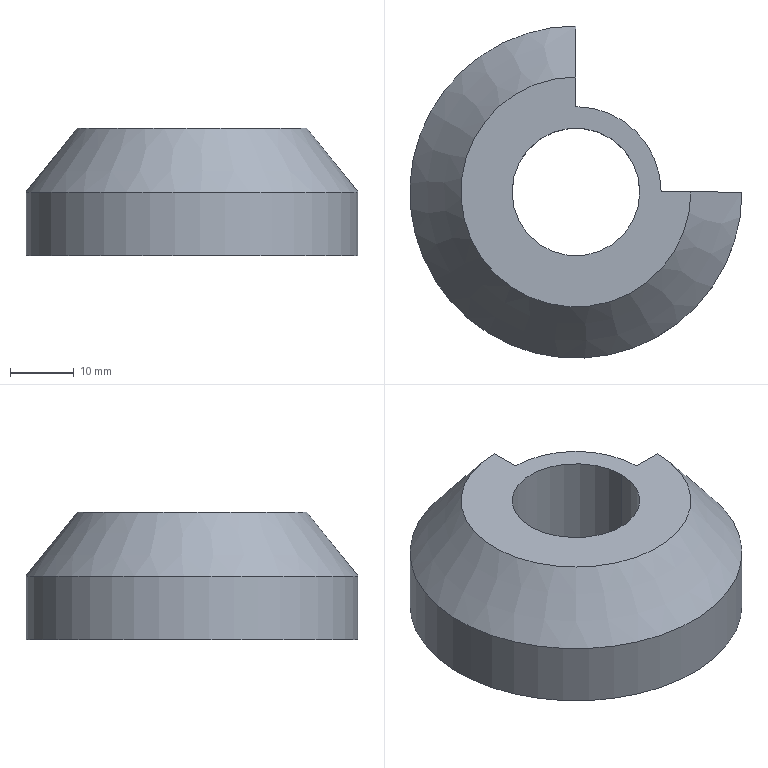Part | STEP file | Twistshift Body3 speed | 1 solid | 9 faces | box 52 x 52 x 20 mm | volume 23974 mm3 | cylinder 4 | plane 4 | cone 1 | commonest cylinder face diameters 20 x2 26.699 x1 52 x1
STEP:
#1=CARTESIAN_POINT('',(0.,0.,0.));
#2=DIRECTION('',(0.,0.,1.));
#3=DIRECTION('',(1.,0.,0.));
#4=AXIS2_PLACEMENT_3D('',#1,#2,#3);
#5=CARTESIAN_POINT('',(10.,0.,20.));
#6=VERTEX_POINT('',#5);
#7=CARTESIAN_POINT('',(10.,0.,0.));
#8=VERTEX_POINT('',#7);
#9=CARTESIAN_POINT('',(10.,0.,-78.017));
#10=DIRECTION('',(0.,0.,-1.));
#11=VECTOR('',#10,1.);
#12=LINE('',#9,#11);
#13=CARTESIAN_POINT('',(0.,0.,-78.017));
#14=DIRECTION('',(0.,0.,-1.));
#15=DIRECTION('',(1.,0.,0.));
#16=AXIS2_PLACEMENT_3D('',#13,#14,#15);
#17=CYLINDRICAL_SURFACE('',#16,10.);
#18=CARTESIAN_POINT('',(6.283,0.));
#19=DIRECTION('',(0.,1.));
#20=VECTOR('',#19,1.);
#21=LINE('',#18,#20);
#22=(GEOMETRIC_REPRESENTATION_CONTEXT(2)PARAMETRIC_REPRESENTATION_CONTEXT()REPRESENTATION_CONTEXT('',''));
#23=DEFINITIONAL_REPRESENTATION('',(#21),#22);
#24=PCURVE('',#17,#23);
#25=CARTESIAN_POINT('',(0.,0.,-78.017));
#26=DIRECTION('',(0.,0.,-1.));
#27=DIRECTION('',(1.,0.,0.));
#28=AXIS2_PLACEMENT_3D('',#25,#26,#27);
#29=CYLINDRICAL_SURFACE('',#28,10.);
#30=CARTESIAN_POINT('',(0.,0.));
#31=DIRECTION('',(0.,1.));
#32=VECTOR('',#31,1.);
#33=LINE('',#30,#32);
#34=(GEOMETRIC_REPRESENTATION_CONTEXT(2)PARAMETRIC_REPRESENTATION_CONTEXT()REPRESENTATION_CONTEXT('',''));
#35=DEFINITIONAL_REPRESENTATION('',(#33),#34);
#36=PCURVE('',#29,#35);
#37=SURFACE_CURVE('',#12,(#24,#36),.PCURVE_S1.);
#38=EDGE_CURVE('',#6,#8,#37,.T.);
#39=ORIENTED_EDGE('',*,*,#38,.T.);
#40=CARTESIAN_POINT('',(-10.,0.,0.));
#41=VERTEX_POINT('',#40);
#42=CARTESIAN_POINT('',(0.,0.,0.));
#43=DIRECTION('',(0.,0.,1.));
#44=DIRECTION('',(1.,0.,0.));
#45=AXIS2_PLACEMENT_3D('',#42,#43,#44);
#46=CIRCLE('',#45,10.);
#47=CARTESIAN_POINT('',(6.283,-78.017));
#48=DIRECTION('',(-1.,0.));
#49=VECTOR('',#48,1.);
#50=LINE('',#47,#49);
#51=(GEOMETRIC_REPRESENTATION_CONTEXT(2)PARAMETRIC_REPRESENTATION_CONTEXT()REPRESENTATION_CONTEXT('',''));
#52=DEFINITIONAL_REPRESENTATION('',(#50),#51);
#53=PCURVE('',#17,#52);
#54=CARTESIAN_POINT('',(0.,10.,0.));
#55=DIRECTION('',(0.,0.,1.));
#56=DIRECTION('',(-1.,0.,0.));
#57=AXIS2_PLACEMENT_3D('',#54,#55,#56);
#58=PLANE('',#57);
#59=CARTESIAN_POINT('',(0.,10.));
#60=DIRECTION('',(-1.,0.));
#61=AXIS2_PLACEMENT_2D('',#59,#60);
#62=CIRCLE('',#61,10.);
#63=(GEOMETRIC_REPRESENTATION_CONTEXT(2)PARAMETRIC_REPRESENTATION_CONTEXT()REPRESENTATION_CONTEXT('',''));
#64=DEFINITIONAL_REPRESENTATION('',(#62),#63);
#65=PCURVE('',#58,#64);
#66=SURFACE_CURVE('',#46,(#53,#65),.PCURVE_S1.);
#67=EDGE_CURVE('',#8,#41,#66,.T.);
#68=ORIENTED_EDGE('',*,*,#67,.T.);
#69=CARTESIAN_POINT('',(-10.,0.,20.));
#70=VERTEX_POINT('',#69);
#71=CARTESIAN_POINT('',(-10.,0.,-78.017));
#72=DIRECTION('',(0.,0.,-1.));
#73=VECTOR('',#72,1.);
#74=LINE('',#71,#73);
#75=CARTESIAN_POINT('',(3.142,0.));
#76=DIRECTION('',(0.,1.));
#77=VECTOR('',#76,1.);
#78=LINE('',#75,#77);
#79=(GEOMETRIC_REPRESENTATION_CONTEXT(2)PARAMETRIC_REPRESENTATION_CONTEXT()REPRESENTATION_CONTEXT('',''));
#80=DEFINITIONAL_REPRESENTATION('',(#78),#79);
#81=PCURVE('',#17,#80);
#82=CARTESIAN_POINT('',(3.142,0.));
#83=DIRECTION('',(0.,1.));
#84=VECTOR('',#83,1.);
#85=LINE('',#82,#84);
#86=(GEOMETRIC_REPRESENTATION_CONTEXT(2)PARAMETRIC_REPRESENTATION_CONTEXT()REPRESENTATION_CONTEXT('',''));
#87=DEFINITIONAL_REPRESENTATION('',(#85),#86);
#88=PCURVE('',#29,#87);
#89=SURFACE_CURVE('',#74,(#81,#88),.PCURVE_S1.);
#90=EDGE_CURVE('',#70,#41,#89,.T.);
#91=ORIENTED_EDGE('',*,*,#90,.F.);
#92=CARTESIAN_POINT('',(0.,0.,20.));
#93=DIRECTION('',(0.,0.,1.));
#94=DIRECTION('',(1.,0.,0.));
#95=AXIS2_PLACEMENT_3D('',#92,#93,#94);
#96=CIRCLE('',#95,10.);
#97=CARTESIAN_POINT('',(6.283,-98.017));
#98=DIRECTION('',(-1.,0.));
#99=VECTOR('',#98,1.);
#100=LINE('',#97,#99);
#101=(GEOMETRIC_REPRESENTATION_CONTEXT(2)PARAMETRIC_REPRESENTATION_CONTEXT()REPRESENTATION_CONTEXT('',''));
#102=DEFINITIONAL_REPRESENTATION('',(#100),#101);
#103=PCURVE('',#17,#102);
#104=CARTESIAN_POINT('',(0.,10.,20.));
#105=DIRECTION('',(0.,0.,-1.));
#106=DIRECTION('',(1.,0.,0.));
#107=AXIS2_PLACEMENT_3D('',#104,#105,#106);
#108=PLANE('',#107);
#109=CARTESIAN_POINT('',(10.,10.));
#110=CARTESIAN_POINT('',(10.,-7.321));
#111=CARTESIAN_POINT('',(-5.,1.34));
#112=CARTESIAN_POINT('',(-20.,10.));
#113=CARTESIAN_POINT('',(-5.,18.66));
#114=CARTESIAN_POINT('',(10.,27.321));
#115=CARTESIAN_POINT('',(10.,10.));
#116=(BOUNDED_CURVE()B_SPLINE_CURVE(2,(#109,#110,#111,#112,#113,#114,#115),.UNSPECIFIED.,.T.,.F.)B_SPLINE_CURVE_WITH_KNOTS((1,2,2,2,2,1),(-2.094,0.,2.094,4.189,6.283,8.378),.UNSPECIFIED.)CURVE()GEOMETRIC_REPRESENTATION_ITEM()RATIONAL_B_SPLINE_CURVE((1.,0.5,1.,0.5,1.,0.5,1.))REPRESENTATION_ITEM(''));
#117=(GEOMETRIC_REPRESENTATION_CONTEXT(2)PARAMETRIC_REPRESENTATION_CONTEXT()REPRESENTATION_CONTEXT('',''));
#118=DEFINITIONAL_REPRESENTATION('',(#116),#117);
#119=PCURVE('',#108,#118);
#120=SURFACE_CURVE('',#96,(#103,#119),.PCURVE_S1.);
#121=EDGE_CURVE('',#6,#70,#120,.T.);
#122=ORIENTED_EDGE('',*,*,#121,.F.);
#123=EDGE_LOOP('',(#39,#68,#91,#122));
#124=FACE_BOUND('',#123,.F.);
#125=ADVANCED_FACE('',(#124),#17,.F.);
#126=CARTESIAN_POINT('',(0.,26.,10.));
#127=VERTEX_POINT('',#126);
#128=CARTESIAN_POINT('',(26.,0.,10.));
#129=VERTEX_POINT('',#128);
#130=CARTESIAN_POINT('',(0.,0.,10.));
#131=DIRECTION('',(0.,0.,1.));
#132=DIRECTION('',(1.,0.,0.));
#133=AXIS2_PLACEMENT_3D('',#130,#131,#132);
#134=CIRCLE('',#133,26.);
#135=CARTESIAN_POINT('',(0.,0.,-78.017));
#136=DIRECTION('',(0.,0.,-1.));
#137=DIRECTION('',(1.,0.,0.));
#138=AXIS2_PLACEMENT_3D('',#135,#136,#137);
#139=CYLINDRICAL_SURFACE('',#138,26.);
#140=CARTESIAN_POINT('',(6.283,-88.017));
#141=DIRECTION('',(-1.,0.));
#142=VECTOR('',#141,1.);
#143=LINE('',#140,#142);
#144=(GEOMETRIC_REPRESENTATION_CONTEXT(2)PARAMETRIC_REPRESENTATION_CONTEXT()REPRESENTATION_CONTEXT('',''));
#145=DEFINITIONAL_REPRESENTATION('',(#143),#144);
#146=PCURVE('',#139,#145);
#147=CARTESIAN_POINT('',(0.,0.,20.));
#148=DIRECTION('',(0.,0.,-1.));
#149=DIRECTION('',(1.,0.,0.));
#150=AXIS2_PLACEMENT_3D('',#147,#148,#149);
#151=CONICAL_SURFACE('',#150,18.,0.6747);
#152=CARTESIAN_POINT('',(6.283,10.));
#153=DIRECTION('',(-1.,0.));
#154=VECTOR('',#153,1.);
#155=LINE('',#152,#154);
#156=(GEOMETRIC_REPRESENTATION_CONTEXT(2)PARAMETRIC_REPRESENTATION_CONTEXT()REPRESENTATION_CONTEXT('',''));
#157=DEFINITIONAL_REPRESENTATION('',(#155),#156);
#158=PCURVE('',#151,#157);
#159=SURFACE_CURVE('',#134,(#146,#158),.PCURVE_S1.);
#160=EDGE_CURVE('',#127,#129,#159,.T.);
#161=ORIENTED_EDGE('',*,*,#160,.F.);
#162=CARTESIAN_POINT('',(0.,26.,0.));
#163=VERTEX_POINT('',#162);
#164=CARTESIAN_POINT('',(0.,26.,0.));
#165=DIRECTION('',(0.,0.,-1.));
#166=VECTOR('',#165,1.);
#167=LINE('',#164,#166);
#168=CARTESIAN_POINT('',(4.712,-78.017));
#169=DIRECTION('',(0.,1.));
#170=VECTOR('',#169,1.);
#171=LINE('',#168,#170);
#172=(GEOMETRIC_REPRESENTATION_CONTEXT(2)PARAMETRIC_REPRESENTATION_CONTEXT()REPRESENTATION_CONTEXT('',''));
#173=DEFINITIONAL_REPRESENTATION('',(#171),#172);
#174=PCURVE('',#139,#173);
#175=CARTESIAN_POINT('',(0.,13.35,0.));
#176=DIRECTION('',(-1.,0.,0.));
#177=DIRECTION('',(0.,0.,-1.));
#178=AXIS2_PLACEMENT_3D('',#175,#176,#177);
#179=PLANE('',#178);
#180=CARTESIAN_POINT('',(0.,-12.65));
#181=DIRECTION('',(1.,0.));
#182=VECTOR('',#181,1.);
#183=LINE('',#180,#182);
#184=(GEOMETRIC_REPRESENTATION_CONTEXT(2)PARAMETRIC_REPRESENTATION_CONTEXT()REPRESENTATION_CONTEXT('',''));
#185=DEFINITIONAL_REPRESENTATION('',(#183),#184);
#186=PCURVE('',#179,#185);
#187=SURFACE_CURVE('',#167,(#174,#186),.PCURVE_S1.);
#188=EDGE_CURVE('',#127,#163,#187,.T.);
#189=ORIENTED_EDGE('',*,*,#188,.T.);
#190=CARTESIAN_POINT('',(26.,0.,0.));
#191=VERTEX_POINT('',#190);
#192=CARTESIAN_POINT('',(0.,0.,0.));
#193=DIRECTION('',(0.,0.,1.));
#194=DIRECTION('',(1.,0.,0.));
#195=AXIS2_PLACEMENT_3D('',#192,#193,#194);
#196=CIRCLE('',#195,26.);
#197=CARTESIAN_POINT('',(6.283,-78.017));
#198=DIRECTION('',(-1.,0.));
#199=VECTOR('',#198,1.);
#200=LINE('',#197,#199);
#201=(GEOMETRIC_REPRESENTATION_CONTEXT(2)PARAMETRIC_REPRESENTATION_CONTEXT()REPRESENTATION_CONTEXT('',''));
#202=DEFINITIONAL_REPRESENTATION('',(#200),#201);
#203=PCURVE('',#139,#202);
#204=CARTESIAN_POINT('',(0.,10.));
#205=DIRECTION('',(-1.,0.));
#206=AXIS2_PLACEMENT_2D('',#204,#205);
#207=CIRCLE('',#206,26.);
#208=(GEOMETRIC_REPRESENTATION_CONTEXT(2)PARAMETRIC_REPRESENTATION_CONTEXT()REPRESENTATION_CONTEXT('',''));
#209=DEFINITIONAL_REPRESENTATION('',(#207),#208);
#210=PCURVE('',#58,#209);
#211=SURFACE_CURVE('',#196,(#203,#210),.PCURVE_S1.);
#212=EDGE_CURVE('',#163,#191,#211,.T.);
#213=ORIENTED_EDGE('',*,*,#212,.T.);
#214=CARTESIAN_POINT('',(26.,0.,-78.017));
#215=DIRECTION('',(0.,0.,-1.));
#216=VECTOR('',#215,1.);
#217=LINE('',#214,#216);
#218=CARTESIAN_POINT('',(0.,0.));
#219=DIRECTION('',(0.,1.));
#220=VECTOR('',#219,1.);
#221=LINE('',#218,#220);
#222=(GEOMETRIC_REPRESENTATION_CONTEXT(2)PARAMETRIC_REPRESENTATION_CONTEXT()REPRESENTATION_CONTEXT('',''));
#223=DEFINITIONAL_REPRESENTATION('',(#221),#222);
#224=PCURVE('',#139,#223);
#225=CARTESIAN_POINT('',(13.35,0.,0.));
#226=DIRECTION('',(0.,-1.,0.));
#227=DIRECTION('',(0.,0.,1.));
#228=AXIS2_PLACEMENT_3D('',#225,#226,#227);
#229=PLANE('',#228);
#230=CARTESIAN_POINT('',(-78.017,-12.65));
#231=DIRECTION('',(-1.,0.));
#232=VECTOR('',#231,1.);
#233=LINE('',#230,#232);
#234=(GEOMETRIC_REPRESENTATION_CONTEXT(2)PARAMETRIC_REPRESENTATION_CONTEXT()REPRESENTATION_CONTEXT('',''));
#235=DEFINITIONAL_REPRESENTATION('',(#233),#234);
#236=PCURVE('',#229,#235);
#237=SURFACE_CURVE('',#217,(#224,#236),.PCURVE_S1.);
#238=EDGE_CURVE('',#129,#191,#237,.T.);
#239=ORIENTED_EDGE('',*,*,#238,.F.);
#240=EDGE_LOOP('',(#161,#189,#213,#239));
#241=FACE_BOUND('',#240,.T.);
#242=ADVANCED_FACE('',(#241),#139,.T.);
#243=CARTESIAN_POINT('',(0.,18.,20.));
#244=VERTEX_POINT('',#243);
#245=CARTESIAN_POINT('',(18.,0.,20.));
#246=VERTEX_POINT('',#245);
#247=CARTESIAN_POINT('',(0.,0.,20.));
#248=DIRECTION('',(0.,0.,1.));
#249=DIRECTION('',(1.,0.,0.));
#250=AXIS2_PLACEMENT_3D('',#247,#248,#249);
#251=CIRCLE('',#250,18.);
#252=CARTESIAN_POINT('',(6.283,0.));
#253=DIRECTION('',(-1.,0.));
#254=VECTOR('',#253,1.);
#255=LINE('',#252,#254);
#256=(GEOMETRIC_REPRESENTATION_CONTEXT(2)PARAMETRIC_REPRESENTATION_CONTEXT()REPRESENTATION_CONTEXT('',''));
#257=DEFINITIONAL_REPRESENTATION('',(#255),#256);
#258=PCURVE('',#151,#257);
#259=CARTESIAN_POINT('',(18.,10.));
#260=CARTESIAN_POINT('',(18.,-21.177));
#261=CARTESIAN_POINT('',(-9.,-5.588));
#262=CARTESIAN_POINT('',(-36.,10.));
#263=CARTESIAN_POINT('',(-9.,25.588));
#264=CARTESIAN_POINT('',(18.,41.177));
#265=CARTESIAN_POINT('',(18.,10.));
#266=(BOUNDED_CURVE()B_SPLINE_CURVE(2,(#259,#260,#261,#262,#263,#264,#265),.UNSPECIFIED.,.T.,.F.)B_SPLINE_CURVE_WITH_KNOTS((1,2,2,2,2,1),(-2.094,0.,2.094,4.189,6.283,8.378),.UNSPECIFIED.)CURVE()GEOMETRIC_REPRESENTATION_ITEM()RATIONAL_B_SPLINE_CURVE((1.,0.5,1.,0.5,1.,0.5,1.))REPRESENTATION_ITEM(''));
#267=(GEOMETRIC_REPRESENTATION_CONTEXT(2)PARAMETRIC_REPRESENTATION_CONTEXT()REPRESENTATION_CONTEXT('',''));
#268=DEFINITIONAL_REPRESENTATION('',(#266),#267);
#269=PCURVE('',#108,#268);
#270=SURFACE_CURVE('',#251,(#258,#269),.PCURVE_S1.);
#271=EDGE_CURVE('',#244,#246,#270,.T.);
#272=ORIENTED_EDGE('',*,*,#271,.F.);
#273=CARTESIAN_POINT('',(0.,26.,10.));
#274=DIRECTION('',(0.,0.6247,-0.7809));
#275=VECTOR('',#274,1.);
#276=LINE('',#273,#275);
#277=CARTESIAN_POINT('',(4.712,10.));
#278=DIRECTION('',(0.,1.));
#279=VECTOR('',#278,1.);
#280=LINE('',#277,#279);
#281=(GEOMETRIC_REPRESENTATION_CONTEXT(2)PARAMETRIC_REPRESENTATION_CONTEXT()REPRESENTATION_CONTEXT('',''));
#282=DEFINITIONAL_REPRESENTATION('',(#280),#281);
#283=PCURVE('',#151,#282);
#284=CARTESIAN_POINT('',(-10.,-12.65));
#285=DIRECTION('',(0.7809,-0.6247));
#286=VECTOR('',#285,1.);
#287=LINE('',#284,#286);
#288=(GEOMETRIC_REPRESENTATION_CONTEXT(2)PARAMETRIC_REPRESENTATION_CONTEXT()REPRESENTATION_CONTEXT('',''));
#289=DEFINITIONAL_REPRESENTATION('',(#287),#288);
#290=PCURVE('',#179,#289);
#291=SURFACE_CURVE('',#276,(#283,#290),.PCURVE_S1.);
#292=EDGE_CURVE('',#244,#127,#291,.T.);
#293=ORIENTED_EDGE('',*,*,#292,.T.);
#294=ORIENTED_EDGE('',*,*,#160,.T.);
#295=CARTESIAN_POINT('',(0.,0.,42.5));
#296=DIRECTION('',(0.6247,0.,-0.7809));
#297=VECTOR('',#296,1.);
#298=LINE('',#295,#297);
#299=CARTESIAN_POINT('',(0.,-22.5));
#300=DIRECTION('',(0.,1.));
#301=VECTOR('',#300,1.);
#302=LINE('',#299,#301);
#303=(GEOMETRIC_REPRESENTATION_CONTEXT(2)PARAMETRIC_REPRESENTATION_CONTEXT()REPRESENTATION_CONTEXT('',''));
#304=DEFINITIONAL_REPRESENTATION('',(#302),#303);
#305=PCURVE('',#151,#304);
#306=CARTESIAN_POINT('',(42.5,13.35));
#307=DIRECTION('',(-0.7809,-0.6247));
#308=VECTOR('',#307,1.);
#309=LINE('',#306,#308);
#310=(GEOMETRIC_REPRESENTATION_CONTEXT(2)PARAMETRIC_REPRESENTATION_CONTEXT()REPRESENTATION_CONTEXT('',''));
#311=DEFINITIONAL_REPRESENTATION('',(#309),#310);
#312=PCURVE('',#229,#311);
#313=SURFACE_CURVE('',#298,(#305,#312),.PCURVE_S1.);
#314=EDGE_CURVE('',#246,#129,#313,.T.);
#315=ORIENTED_EDGE('',*,*,#314,.F.);
#316=EDGE_LOOP('',(#272,#293,#294,#315));
#317=FACE_BOUND('',#316,.T.);
#318=ADVANCED_FACE('',(#317),#151,.T.);
#319=ORIENTED_EDGE('',*,*,#121,.F.);
#320=CARTESIAN_POINT('',(0.,0.,20.));
#321=DIRECTION('',(0.,0.,1.));
#322=DIRECTION('',(1.,0.,0.));
#323=AXIS2_PLACEMENT_3D('',#320,#321,#322);
#324=CIRCLE('',#323,10.);
#325=CARTESIAN_POINT('',(10.,10.));
#326=CARTESIAN_POINT('',(10.,-7.321));
#327=CARTESIAN_POINT('',(-5.,1.34));
#328=CARTESIAN_POINT('',(-20.,10.));
#329=CARTESIAN_POINT('',(-5.,18.66));
#330=CARTESIAN_POINT('',(10.,27.321));
#331=CARTESIAN_POINT('',(10.,10.));
#332=(BOUNDED_CURVE()B_SPLINE_CURVE(2,(#325,#326,#327,#328,#329,#330,#331),.UNSPECIFIED.,.T.,.F.)B_SPLINE_CURVE_WITH_KNOTS((1,2,2,2,2,1),(-2.094,0.,2.094,4.189,6.283,8.378),.UNSPECIFIED.)CURVE()GEOMETRIC_REPRESENTATION_ITEM()RATIONAL_B_SPLINE_CURVE((1.,0.5,1.,0.5,1.,0.5,1.))REPRESENTATION_ITEM(''));
#333=(GEOMETRIC_REPRESENTATION_CONTEXT(2)PARAMETRIC_REPRESENTATION_CONTEXT()REPRESENTATION_CONTEXT('',''));
#334=DEFINITIONAL_REPRESENTATION('',(#332),#333);
#335=PCURVE('',#108,#334);
#336=CARTESIAN_POINT('',(6.283,-98.017));
#337=DIRECTION('',(-1.,0.));
#338=VECTOR('',#337,1.);
#339=LINE('',#336,#338);
#340=(GEOMETRIC_REPRESENTATION_CONTEXT(2)PARAMETRIC_REPRESENTATION_CONTEXT()REPRESENTATION_CONTEXT('',''));
#341=DEFINITIONAL_REPRESENTATION('',(#339),#340);
#342=PCURVE('',#29,#341);
#343=SURFACE_CURVE('',#324,(#335,#342),.PCURVE_S1.);
#344=EDGE_CURVE('',#70,#6,#343,.T.);
#345=ORIENTED_EDGE('',*,*,#344,.F.);
#346=EDGE_LOOP('',(#319,#345));
#347=FACE_BOUND('',#346,.T.);
#348=ORIENTED_EDGE('',*,*,#271,.T.);
#349=CARTESIAN_POINT('',(13.35,0.,20.));
#350=VERTEX_POINT('',#349);
#351=CARTESIAN_POINT('',(0.,0.,20.));
#352=DIRECTION('',(1.,0.,0.));
#353=VECTOR('',#352,1.);
#354=LINE('',#351,#353);
#355=CARTESIAN_POINT('',(0.,10.));
#356=DIRECTION('',(1.,0.));
#357=VECTOR('',#356,1.);
#358=LINE('',#355,#357);
#359=(GEOMETRIC_REPRESENTATION_CONTEXT(2)PARAMETRIC_REPRESENTATION_CONTEXT()REPRESENTATION_CONTEXT('',''));
#360=DEFINITIONAL_REPRESENTATION('',(#358),#359);
#361=PCURVE('',#108,#360);
#362=CARTESIAN_POINT('',(20.,13.35));
#363=DIRECTION('',(0.,-1.));
#364=VECTOR('',#363,1.);
#365=LINE('',#362,#364);
#366=(GEOMETRIC_REPRESENTATION_CONTEXT(2)PARAMETRIC_REPRESENTATION_CONTEXT()REPRESENTATION_CONTEXT('',''));
#367=DEFINITIONAL_REPRESENTATION('',(#365),#366);
#368=PCURVE('',#229,#367);
#369=SURFACE_CURVE('',#354,(#361,#368),.PCURVE_S1.);
#370=EDGE_CURVE('',#350,#246,#369,.T.);
#371=ORIENTED_EDGE('',*,*,#370,.F.);
#372=CARTESIAN_POINT('',(0.,13.35,20.));
#373=VERTEX_POINT('',#372);
#374=CARTESIAN_POINT('',(0.,0.,20.));
#375=DIRECTION('',(0.,0.,-1.));
#376=DIRECTION('',(1.,0.,0.));
#377=AXIS2_PLACEMENT_3D('',#374,#375,#376);
#378=CIRCLE('',#377,13.35);
#379=CARTESIAN_POINT('',(0.,10.));
#380=DIRECTION('',(1.,0.));
#381=AXIS2_PLACEMENT_2D('',#379,#380);
#382=CIRCLE('',#381,13.35);
#383=(GEOMETRIC_REPRESENTATION_CONTEXT(2)PARAMETRIC_REPRESENTATION_CONTEXT()REPRESENTATION_CONTEXT('',''));
#384=DEFINITIONAL_REPRESENTATION('',(#382),#383);
#385=PCURVE('',#108,#384);
#386=CARTESIAN_POINT('',(0.,0.,0.));
#387=DIRECTION('',(0.,0.,1.));
#388=DIRECTION('',(-1.,0.,0.));
#389=AXIS2_PLACEMENT_3D('',#386,#387,#388);
#390=CYLINDRICAL_SURFACE('',#389,13.35);
#391=CARTESIAN_POINT('',(9.425,20.));
#392=DIRECTION('',(-1.,0.));
#393=VECTOR('',#392,1.);
#394=LINE('',#391,#393);
#395=(GEOMETRIC_REPRESENTATION_CONTEXT(2)PARAMETRIC_REPRESENTATION_CONTEXT()REPRESENTATION_CONTEXT('',''));
#396=DEFINITIONAL_REPRESENTATION('',(#394),#395);
#397=PCURVE('',#390,#396);
#398=SURFACE_CURVE('',#378,(#385,#397),.PCURVE_S1.);
#399=EDGE_CURVE('',#373,#350,#398,.T.);
#400=ORIENTED_EDGE('',*,*,#399,.F.);
#401=CARTESIAN_POINT('',(0.,10.,20.));
#402=DIRECTION('',(0.,-1.,0.));
#403=VECTOR('',#402,1.);
#404=LINE('',#401,#403);
#405=CARTESIAN_POINT('',(0.,0.));
#406=DIRECTION('',(0.,1.));
#407=VECTOR('',#406,1.);
#408=LINE('',#405,#407);
#409=(GEOMETRIC_REPRESENTATION_CONTEXT(2)PARAMETRIC_REPRESENTATION_CONTEXT()REPRESENTATION_CONTEXT('',''));
#410=DEFINITIONAL_REPRESENTATION('',(#408),#409);
#411=PCURVE('',#108,#410);
#412=CARTESIAN_POINT('',(-20.,3.35));
#413=DIRECTION('',(0.,1.));
#414=VECTOR('',#413,1.);
#415=LINE('',#412,#414);
#416=(GEOMETRIC_REPRESENTATION_CONTEXT(2)PARAMETRIC_REPRESENTATION_CONTEXT()REPRESENTATION_CONTEXT('',''));
#417=DEFINITIONAL_REPRESENTATION('',(#415),#416);
#418=PCURVE('',#179,#417);
#419=SURFACE_CURVE('',#404,(#411,#418),.PCURVE_S1.);
#420=EDGE_CURVE('',#244,#373,#419,.T.);
#421=ORIENTED_EDGE('',*,*,#420,.F.);
#422=EDGE_LOOP('',(#348,#371,#400,#421));
#423=FACE_BOUND('',#422,.T.);
#424=ADVANCED_FACE('',(#347,#423),#108,.F.);
#425=CARTESIAN_POINT('',(13.35,0.,0.));
#426=VERTEX_POINT('',#425);
#427=CARTESIAN_POINT('',(0.,13.35,0.));
#428=VERTEX_POINT('',#427);
#429=CARTESIAN_POINT('',(0.,0.,0.));
#430=DIRECTION('',(0.,0.,1.));
#431=DIRECTION('',(-1.,0.,0.));
#432=AXIS2_PLACEMENT_3D('',#429,#430,#431);
#433=CIRCLE('',#432,13.35);
#434=CARTESIAN_POINT('',(0.,10.));
#435=DIRECTION('',(1.,0.));
#436=AXIS2_PLACEMENT_2D('',#434,#435);
#437=CIRCLE('',#436,13.35);
#438=(GEOMETRIC_REPRESENTATION_CONTEXT(2)PARAMETRIC_REPRESENTATION_CONTEXT()REPRESENTATION_CONTEXT('',''));
#439=DEFINITIONAL_REPRESENTATION('',(#437),#438);
#440=PCURVE('',#58,#439);
#441=CARTESIAN_POINT('',(0.,0.));
#442=DIRECTION('',(1.,0.));
#443=VECTOR('',#442,1.);
#444=LINE('',#441,#443);
#445=(GEOMETRIC_REPRESENTATION_CONTEXT(2)PARAMETRIC_REPRESENTATION_CONTEXT()REPRESENTATION_CONTEXT('',''));
#446=DEFINITIONAL_REPRESENTATION('',(#444),#445);
#447=PCURVE('',#390,#446);
#448=SURFACE_CURVE('',#433,(#440,#447),.PCURVE_S1.);
#449=EDGE_CURVE('',#426,#428,#448,.T.);
#450=ORIENTED_EDGE('',*,*,#449,.F.);
#451=CARTESIAN_POINT('',(13.35,0.,0.));
#452=DIRECTION('',(-1.,0.,0.));
#453=VECTOR('',#452,1.);
#454=LINE('',#451,#453);
#455=CARTESIAN_POINT('',(-13.35,10.));
#456=DIRECTION('',(1.,0.));
#457=VECTOR('',#456,1.);
#458=LINE('',#455,#457);
#459=(GEOMETRIC_REPRESENTATION_CONTEXT(2)PARAMETRIC_REPRESENTATION_CONTEXT()REPRESENTATION_CONTEXT('',''));
#460=DEFINITIONAL_REPRESENTATION('',(#458),#459);
#461=PCURVE('',#58,#460);
#462=CARTESIAN_POINT('',(0.,0.));
#463=DIRECTION('',(0.,1.));
#464=VECTOR('',#463,1.);
#465=LINE('',#462,#464);
#466=(GEOMETRIC_REPRESENTATION_CONTEXT(2)PARAMETRIC_REPRESENTATION_CONTEXT()REPRESENTATION_CONTEXT('',''));
#467=DEFINITIONAL_REPRESENTATION('',(#465),#466);
#468=PCURVE('',#229,#467);
#469=SURFACE_CURVE('',#454,(#461,#468),.PCURVE_S1.);
#470=EDGE_CURVE('',#191,#426,#469,.T.);
#471=ORIENTED_EDGE('',*,*,#470,.F.);
#472=ORIENTED_EDGE('',*,*,#212,.F.);
#473=CARTESIAN_POINT('',(0.,13.35,0.));
#474=DIRECTION('',(0.,1.,0.));
#475=VECTOR('',#474,1.);
#476=LINE('',#473,#475);
#477=CARTESIAN_POINT('',(0.,-3.35));
#478=DIRECTION('',(0.,-1.));
#479=VECTOR('',#478,1.);
#480=LINE('',#477,#479);
#481=(GEOMETRIC_REPRESENTATION_CONTEXT(2)PARAMETRIC_REPRESENTATION_CONTEXT()REPRESENTATION_CONTEXT('',''));
#482=DEFINITIONAL_REPRESENTATION('',(#480),#481);
#483=PCURVE('',#58,#482);
#484=CARTESIAN_POINT('',(0.,0.));
#485=DIRECTION('',(0.,-1.));
#486=VECTOR('',#485,1.);
#487=LINE('',#484,#486);
#488=(GEOMETRIC_REPRESENTATION_CONTEXT(2)PARAMETRIC_REPRESENTATION_CONTEXT()REPRESENTATION_CONTEXT('',''));
#489=DEFINITIONAL_REPRESENTATION('',(#487),#488);
#490=PCURVE('',#179,#489);
#491=SURFACE_CURVE('',#476,(#483,#490),.PCURVE_S1.);
#492=EDGE_CURVE('',#428,#163,#491,.T.);
#493=ORIENTED_EDGE('',*,*,#492,.F.);
#494=EDGE_LOOP('',(#450,#471,#472,#493));
#495=FACE_BOUND('',#494,.T.);
#496=ORIENTED_EDGE('',*,*,#67,.T.);
#497=CARTESIAN_POINT('',(0.,0.,0.));
#498=DIRECTION('',(0.,0.,1.));
#499=DIRECTION('',(1.,0.,0.));
#500=AXIS2_PLACEMENT_3D('',#497,#498,#499);
#501=CIRCLE('',#500,10.);
#502=CARTESIAN_POINT('',(0.,10.));
#503=DIRECTION('',(-1.,0.));
#504=AXIS2_PLACEMENT_2D('',#502,#503);
#505=CIRCLE('',#504,10.);
#506=(GEOMETRIC_REPRESENTATION_CONTEXT(2)PARAMETRIC_REPRESENTATION_CONTEXT()REPRESENTATION_CONTEXT('',''));
#507=DEFINITIONAL_REPRESENTATION('',(#505),#506);
#508=PCURVE('',#58,#507);
#509=CARTESIAN_POINT('',(6.283,-78.017));
#510=DIRECTION('',(-1.,0.));
#511=VECTOR('',#510,1.);
#512=LINE('',#509,#511);
#513=(GEOMETRIC_REPRESENTATION_CONTEXT(2)PARAMETRIC_REPRESENTATION_CONTEXT()REPRESENTATION_CONTEXT('',''));
#514=DEFINITIONAL_REPRESENTATION('',(#512),#513);
#515=PCURVE('',#29,#514);
#516=SURFACE_CURVE('',#501,(#508,#515),.PCURVE_S1.);
#517=EDGE_CURVE('',#41,#8,#516,.T.);
#518=ORIENTED_EDGE('',*,*,#517,.T.);
#519=EDGE_LOOP('',(#496,#518));
#520=FACE_BOUND('',#519,.T.);
#521=ADVANCED_FACE('',(#495,#520),#58,.F.);
#522=ORIENTED_EDGE('',*,*,#517,.T.);
#523=ORIENTED_EDGE('',*,*,#38,.F.);
#524=ORIENTED_EDGE('',*,*,#344,.F.);
#525=ORIENTED_EDGE('',*,*,#90,.T.);
#526=EDGE_LOOP('',(#522,#523,#524,#525));
#527=FACE_BOUND('',#526,.F.);
#528=ADVANCED_FACE('',(#527),#29,.F.);
#529=CARTESIAN_POINT('',(0.,13.35,0.));
#530=DIRECTION('',(0.,0.,1.));
#531=VECTOR('',#530,1.);
#532=LINE('',#529,#531);
#533=CARTESIAN_POINT('',(4.712,0.));
#534=DIRECTION('',(0.,1.));
#535=VECTOR('',#534,1.);
#536=LINE('',#533,#535);
#537=(GEOMETRIC_REPRESENTATION_CONTEXT(2)PARAMETRIC_REPRESENTATION_CONTEXT()REPRESENTATION_CONTEXT('',''));
#538=DEFINITIONAL_REPRESENTATION('',(#536),#537);
#539=PCURVE('',#390,#538);
#540=CARTESIAN_POINT('',(0.,0.));
#541=DIRECTION('',(-1.,0.));
#542=VECTOR('',#541,1.);
#543=LINE('',#540,#542);
#544=(GEOMETRIC_REPRESENTATION_CONTEXT(2)PARAMETRIC_REPRESENTATION_CONTEXT()REPRESENTATION_CONTEXT('',''));
#545=DEFINITIONAL_REPRESENTATION('',(#543),#544);
#546=PCURVE('',#179,#545);
#547=SURFACE_CURVE('',#532,(#539,#546),.PCURVE_S1.);
#548=EDGE_CURVE('',#428,#373,#547,.T.);
#549=ORIENTED_EDGE('',*,*,#548,.T.);
#550=ORIENTED_EDGE('',*,*,#399,.T.);
#551=CARTESIAN_POINT('',(13.35,0.,0.));
#552=DIRECTION('',(0.,0.,1.));
#553=VECTOR('',#552,1.);
#554=LINE('',#551,#553);
#555=CARTESIAN_POINT('',(3.142,0.));
#556=DIRECTION('',(0.,1.));
#557=VECTOR('',#556,1.);
#558=LINE('',#555,#557);
#559=(GEOMETRIC_REPRESENTATION_CONTEXT(2)PARAMETRIC_REPRESENTATION_CONTEXT()REPRESENTATION_CONTEXT('',''));
#560=DEFINITIONAL_REPRESENTATION('',(#558),#559);
#561=PCURVE('',#390,#560);
#562=CARTESIAN_POINT('',(0.,0.));
#563=DIRECTION('',(1.,0.));
#564=VECTOR('',#563,1.);
#565=LINE('',#562,#564);
#566=(GEOMETRIC_REPRESENTATION_CONTEXT(2)PARAMETRIC_REPRESENTATION_CONTEXT()REPRESENTATION_CONTEXT('',''));
#567=DEFINITIONAL_REPRESENTATION('',(#565),#566);
#568=PCURVE('',#229,#567);
#569=SURFACE_CURVE('',#554,(#561,#568),.PCURVE_S1.);
#570=EDGE_CURVE('',#426,#350,#569,.T.);
#571=ORIENTED_EDGE('',*,*,#570,.F.);
#572=ORIENTED_EDGE('',*,*,#449,.T.);
#573=EDGE_LOOP('',(#549,#550,#571,#572));
#574=FACE_BOUND('',#573,.T.);
#575=ADVANCED_FACE('',(#574),#390,.T.);
#576=ORIENTED_EDGE('',*,*,#314,.T.);
#577=ORIENTED_EDGE('',*,*,#238,.T.);
#578=ORIENTED_EDGE('',*,*,#470,.T.);
#579=ORIENTED_EDGE('',*,*,#570,.T.);
#580=ORIENTED_EDGE('',*,*,#370,.T.);
#581=EDGE_LOOP('',(#576,#577,#578,#579,#580));
#582=FACE_BOUND('',#581,.T.);
#583=ADVANCED_FACE('',(#582),#229,.F.);
#584=ORIENTED_EDGE('',*,*,#292,.F.);
#585=ORIENTED_EDGE('',*,*,#420,.T.);
#586=ORIENTED_EDGE('',*,*,#548,.F.);
#587=ORIENTED_EDGE('',*,*,#492,.T.);
#588=ORIENTED_EDGE('',*,*,#188,.F.);
#589=EDGE_LOOP('',(#584,#585,#586,#587,#588));
#590=FACE_BOUND('',#589,.T.);
#591=ADVANCED_FACE('',(#590),#179,.F.);
#592=CLOSED_SHELL('',(#125,#242,#318,#424,#521,#528,#575,#583,#591));
#593=MANIFOLD_SOLID_BREP('',#592);
#594=(LENGTH_UNIT()NAMED_UNIT(*)SI_UNIT(.MILLI.,.METRE.));
#595=UNCERTAINTY_MEASURE_WITH_UNIT(LENGTH_MEASURE(0.0000001),#594,'','');
#596=(NAMED_UNIT(*)PLANE_ANGLE_UNIT()SI_UNIT($,.RADIAN.));
#597=(NAMED_UNIT(*)SI_UNIT($,.STERADIAN.)SOLID_ANGLE_UNIT());
#598=(GEOMETRIC_REPRESENTATION_CONTEXT(3)GLOBAL_UNCERTAINTY_ASSIGNED_CONTEXT((#595))GLOBAL_UNIT_ASSIGNED_CONTEXT((#594,#596,#597))REPRESENTATION_CONTEXT('',''));
#599=ADVANCED_BREP_SHAPE_REPRESENTATION('',(#4,#593),#598);